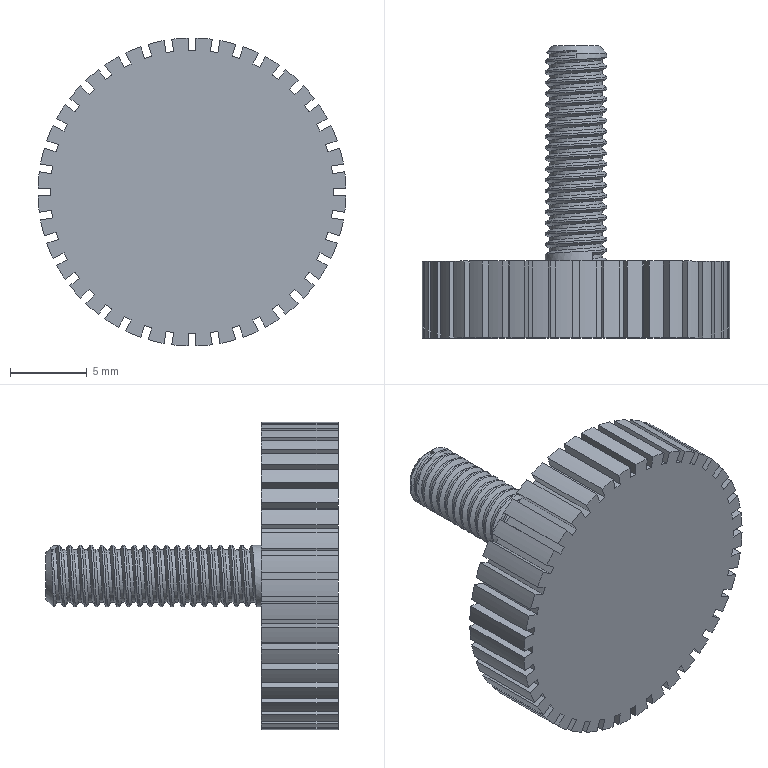Part | NX | features DATUM_CSYS 3, SKETCH 2, CHAMFER 1, DATUM_PLANE 1, EXTRUDE 1, SWP104 1, THREADS 1 | 1 solid | 171 faces | box 19.994 x 19 x 19.994 mm | volume 1639 mm3 | plane 125 | cylinder 42 | spline 3 | cone 1 | commonest cylinder face diameters 20 x40 3.4 x1 4 x1